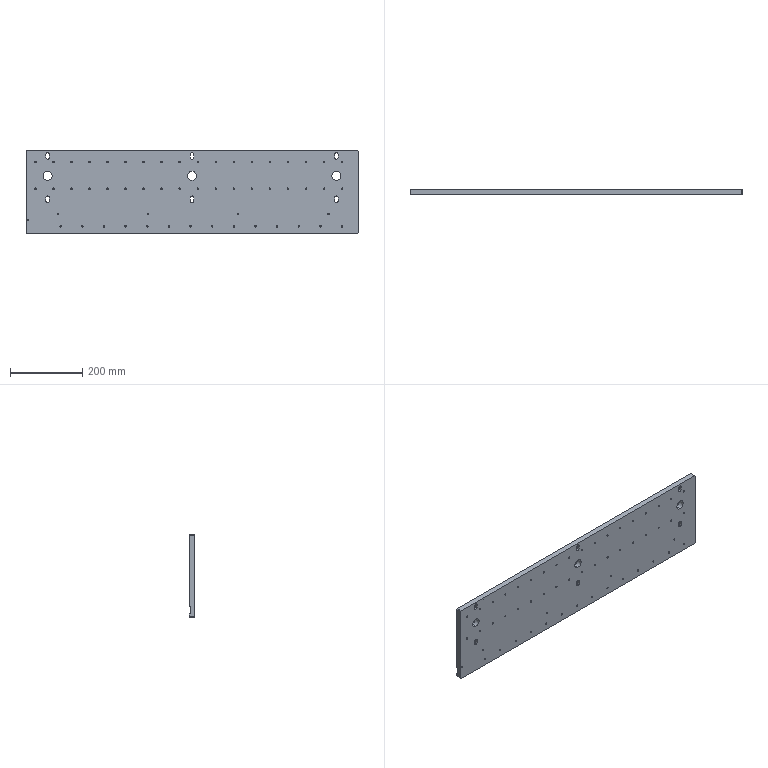Part | NX | features BREP 1 | 1 solid | 220 faces | box 920 x 15 x 230 mm | volume 3081612 mm3 | cylinder 164 | plane 44 | cone 12 | commonest cylinder face diameters 4.2 x110 10 x18 15 x18 3.3 x12 25 x6